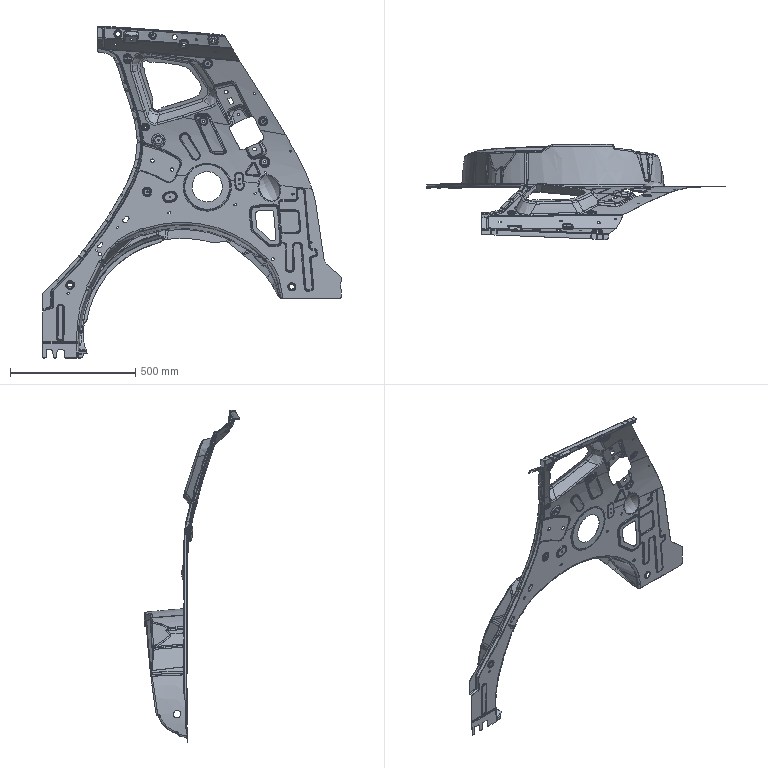Part | STEP file | FNA5401812 | 1 solid | 2309 faces | box 1194 x 381.773 x 1328 mm | volume 686695 mm3 | spline 1861 | cylinder 239 | plane 93 | other 60 | torus 44 | sphere 12 | commonest cylinder face diameters 10 x32 8.4 x28 16 x23 14.4 x19 8 x17 6 x13